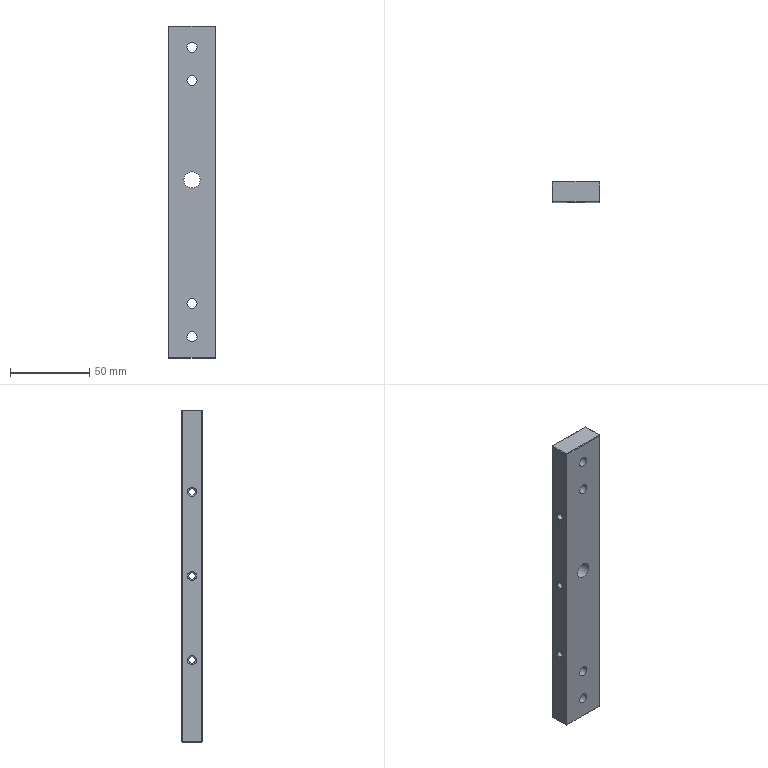Part | NX | 1 solid | 72 faces | box 30 x 13 x 210 mm | volume 76168 mm3 | cylinder 36 | plane 22 | cone 14 | commonest cylinder face diameters 4.2 x18 6.5 x8 11 x8 10.2 x2